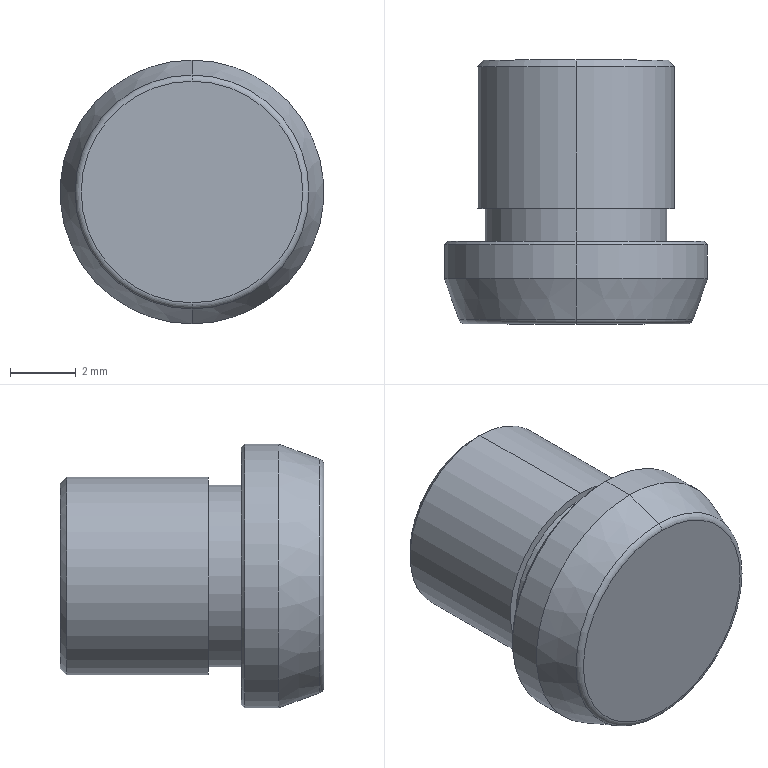Part | STEP file | BPSP-L-03 Fixture Locating Pin_Default | 1 solid | 18 faces | box 8 x 8 x 8 mm | volume 267.813 mm3 | cylinder 6 | cone 6 | plane 4 | torus 2 | commonest cylinder face diameters 5.5 x2 6 x2 8 x2
STEP:
#1=CARTESIAN_POINT('',(0.,0.,0.));
#2=DIRECTION('',(0.,0.,1.));
#3=DIRECTION('',(1.,0.,0.));
#4=AXIS2_PLACEMENT_3D('',#1,#2,#3);
#5=CARTESIAN_POINT('',(0.,7.8,-3.));
#6=VERTEX_POINT('',#5);
#7=CARTESIAN_POINT('',(0.,7.8,3.));
#8=VERTEX_POINT('',#7);
#9=CARTESIAN_POINT('',(0.,7.8,0.));
#10=DIRECTION('',(0.,-1.,0.));
#11=DIRECTION('',(0.,0.,1.));
#12=AXIS2_PLACEMENT_3D('',#9,#10,#11);
#13=CIRCLE('',#12,3.);
#14=CARTESIAN_POINT('',(0.,8.,0.));
#15=DIRECTION('',(0.,-1.,0.));
#16=DIRECTION('',(0.,0.,-1.));
#17=AXIS2_PLACEMENT_3D('',#14,#15,#16);
#18=CYLINDRICAL_SURFACE('',#17,3.);
#19=CARTESIAN_POINT('',(-3.142,0.2));
#20=DIRECTION('',(1.,0.));
#21=VECTOR('',#20,1.);
#22=LINE('',#19,#21);
#23=(GEOMETRIC_REPRESENTATION_CONTEXT(2)PARAMETRIC_REPRESENTATION_CONTEXT()REPRESENTATION_CONTEXT('',''));
#24=DEFINITIONAL_REPRESENTATION('',(#22),#23);
#25=PCURVE('',#18,#24);
#26=CARTESIAN_POINT('',(0.,8.,0.));
#27=DIRECTION('',(0.,-1.,0.));
#28=DIRECTION('',(0.,0.,-1.));
#29=AXIS2_PLACEMENT_3D('',#26,#27,#28);
#30=CONICAL_SURFACE('',#29,2.8,0.7854);
#31=CARTESIAN_POINT('',(-3.142,0.2));
#32=DIRECTION('',(1.,0.));
#33=VECTOR('',#32,1.);
#34=LINE('',#31,#33);
#35=(GEOMETRIC_REPRESENTATION_CONTEXT(2)PARAMETRIC_REPRESENTATION_CONTEXT()REPRESENTATION_CONTEXT('',''));
#36=DEFINITIONAL_REPRESENTATION('',(#34),#35);
#37=PCURVE('',#30,#36);
#38=SURFACE_CURVE('',#13,(#25,#37),.PCURVE_S1.);
#39=EDGE_CURVE('',#6,#8,#38,.T.);
#40=ORIENTED_EDGE('',*,*,#39,.T.);
#41=CARTESIAN_POINT('',(0.,3.5,3.));
#42=VERTEX_POINT('',#41);
#43=CARTESIAN_POINT('',(0.,8.,3.));
#44=DIRECTION('',(0.,-1.,0.));
#45=VECTOR('',#44,1.);
#46=LINE('',#43,#45);
#47=CARTESIAN_POINT('',(3.142,0.));
#48=DIRECTION('',(0.,1.));
#49=VECTOR('',#48,1.);
#50=LINE('',#47,#49);
#51=(GEOMETRIC_REPRESENTATION_CONTEXT(2)PARAMETRIC_REPRESENTATION_CONTEXT()REPRESENTATION_CONTEXT('',''));
#52=DEFINITIONAL_REPRESENTATION('',(#50),#51);
#53=PCURVE('',#18,#52);
#54=CARTESIAN_POINT('',(0.,8.,0.));
#55=DIRECTION('',(0.,-1.,0.));
#56=DIRECTION('',(0.,0.,-1.));
#57=AXIS2_PLACEMENT_3D('',#54,#55,#56);
#58=CYLINDRICAL_SURFACE('',#57,3.);
#59=CARTESIAN_POINT('',(3.142,0.));
#60=DIRECTION('',(0.,1.));
#61=VECTOR('',#60,1.);
#62=LINE('',#59,#61);
#63=(GEOMETRIC_REPRESENTATION_CONTEXT(2)PARAMETRIC_REPRESENTATION_CONTEXT()REPRESENTATION_CONTEXT('',''));
#64=DEFINITIONAL_REPRESENTATION('',(#62),#63);
#65=PCURVE('',#58,#64);
#66=SURFACE_CURVE('',#46,(#53,#65),.PCURVE_S1.);
#67=EDGE_CURVE('',#8,#42,#66,.T.);
#68=ORIENTED_EDGE('',*,*,#67,.T.);
#69=CARTESIAN_POINT('',(0.,3.5,-3.));
#70=VERTEX_POINT('',#69);
#71=CARTESIAN_POINT('',(0.,3.5,0.));
#72=DIRECTION('',(0.,1.,0.));
#73=DIRECTION('',(0.,0.,1.));
#74=AXIS2_PLACEMENT_3D('',#71,#72,#73);
#75=CIRCLE('',#74,3.);
#76=CARTESIAN_POINT('',(3.142,4.5));
#77=DIRECTION('',(-1.,0.));
#78=VECTOR('',#77,1.);
#79=LINE('',#76,#78);
#80=(GEOMETRIC_REPRESENTATION_CONTEXT(2)PARAMETRIC_REPRESENTATION_CONTEXT()REPRESENTATION_CONTEXT('',''));
#81=DEFINITIONAL_REPRESENTATION('',(#79),#80);
#82=PCURVE('',#18,#81);
#83=CARTESIAN_POINT('',(0.,3.5,0.));
#84=DIRECTION('',(0.,1.,0.));
#85=DIRECTION('',(0.,0.,1.));
#86=AXIS2_PLACEMENT_3D('',#83,#84,#85);
#87=PLANE('',#86);
#88=CARTESIAN_POINT('',(0.,0.));
#89=DIRECTION('',(1.,0.));
#90=AXIS2_PLACEMENT_2D('',#88,#89);
#91=CIRCLE('',#90,3.);
#92=(GEOMETRIC_REPRESENTATION_CONTEXT(2)PARAMETRIC_REPRESENTATION_CONTEXT()REPRESENTATION_CONTEXT('',''));
#93=DEFINITIONAL_REPRESENTATION('',(#91),#92);
#94=PCURVE('',#87,#93);
#95=SURFACE_CURVE('',#75,(#82,#94),.PCURVE_S1.);
#96=EDGE_CURVE('',#42,#70,#95,.T.);
#97=ORIENTED_EDGE('',*,*,#96,.T.);
#98=CARTESIAN_POINT('',(0.,8.,-3.));
#99=DIRECTION('',(0.,-1.,0.));
#100=VECTOR('',#99,1.);
#101=LINE('',#98,#100);
#102=CARTESIAN_POINT('',(0.,0.));
#103=DIRECTION('',(0.,1.));
#104=VECTOR('',#103,1.);
#105=LINE('',#102,#104);
#106=(GEOMETRIC_REPRESENTATION_CONTEXT(2)PARAMETRIC_REPRESENTATION_CONTEXT()REPRESENTATION_CONTEXT('',''));
#107=DEFINITIONAL_REPRESENTATION('',(#105),#106);
#108=PCURVE('',#18,#107);
#109=CARTESIAN_POINT('',(6.283,0.));
#110=DIRECTION('',(0.,1.));
#111=VECTOR('',#110,1.);
#112=LINE('',#109,#111);
#113=(GEOMETRIC_REPRESENTATION_CONTEXT(2)PARAMETRIC_REPRESENTATION_CONTEXT()REPRESENTATION_CONTEXT('',''));
#114=DEFINITIONAL_REPRESENTATION('',(#112),#113);
#115=PCURVE('',#58,#114);
#116=SURFACE_CURVE('',#101,(#108,#115),.PCURVE_S1.);
#117=EDGE_CURVE('',#6,#70,#116,.T.);
#118=ORIENTED_EDGE('',*,*,#117,.F.);
#119=EDGE_LOOP('',(#40,#68,#97,#118));
#120=FACE_BOUND('',#119,.T.);
#121=ADVANCED_FACE('',(#120),#18,.T.);
#122=CARTESIAN_POINT('',(0.,8.,2.8));
#123=VERTEX_POINT('',#122);
#124=CARTESIAN_POINT('',(0.,8.,-2.8));
#125=VERTEX_POINT('',#124);
#126=CARTESIAN_POINT('',(0.,8.,0.));
#127=DIRECTION('',(0.,1.,0.));
#128=DIRECTION('',(0.,0.,1.));
#129=AXIS2_PLACEMENT_3D('',#126,#127,#128);
#130=CIRCLE('',#129,2.8);
#131=CARTESIAN_POINT('',(3.142,0.));
#132=DIRECTION('',(-1.,0.));
#133=VECTOR('',#132,1.);
#134=LINE('',#131,#133);
#135=(GEOMETRIC_REPRESENTATION_CONTEXT(2)PARAMETRIC_REPRESENTATION_CONTEXT()REPRESENTATION_CONTEXT('',''));
#136=DEFINITIONAL_REPRESENTATION('',(#134),#135);
#137=PCURVE('',#30,#136);
#138=CARTESIAN_POINT('',(0.,8.,0.));
#139=DIRECTION('',(0.,1.,0.));
#140=DIRECTION('',(0.,0.,1.));
#141=AXIS2_PLACEMENT_3D('',#138,#139,#140);
#142=PLANE('',#141);
#143=CARTESIAN_POINT('',(0.,0.));
#144=DIRECTION('',(1.,0.));
#145=AXIS2_PLACEMENT_2D('',#143,#144);
#146=CIRCLE('',#145,2.8);
#147=(GEOMETRIC_REPRESENTATION_CONTEXT(2)PARAMETRIC_REPRESENTATION_CONTEXT()REPRESENTATION_CONTEXT('',''));
#148=DEFINITIONAL_REPRESENTATION('',(#146),#147);
#149=PCURVE('',#142,#148);
#150=SURFACE_CURVE('',#130,(#137,#149),.PCURVE_S1.);
#151=EDGE_CURVE('',#123,#125,#150,.T.);
#152=ORIENTED_EDGE('',*,*,#151,.F.);
#153=CARTESIAN_POINT('',(0.,8.,2.8));
#154=DIRECTION('',(0.,-0.7071,0.7071));
#155=VECTOR('',#154,1.);
#156=LINE('',#153,#155);
#157=CARTESIAN_POINT('',(3.142,0.));
#158=DIRECTION('',(0.,1.));
#159=VECTOR('',#158,1.);
#160=LINE('',#157,#159);
#161=(GEOMETRIC_REPRESENTATION_CONTEXT(2)PARAMETRIC_REPRESENTATION_CONTEXT()REPRESENTATION_CONTEXT('',''));
#162=DEFINITIONAL_REPRESENTATION('',(#160),#161);
#163=PCURVE('',#30,#162);
#164=CARTESIAN_POINT('',(0.,8.,0.));
#165=DIRECTION('',(0.,-1.,0.));
#166=DIRECTION('',(0.,0.,-1.));
#167=AXIS2_PLACEMENT_3D('',#164,#165,#166);
#168=CONICAL_SURFACE('',#167,2.8,0.7854);
#169=CARTESIAN_POINT('',(3.142,0.));
#170=DIRECTION('',(0.,1.));
#171=VECTOR('',#170,1.);
#172=LINE('',#169,#171);
#173=(GEOMETRIC_REPRESENTATION_CONTEXT(2)PARAMETRIC_REPRESENTATION_CONTEXT()REPRESENTATION_CONTEXT('',''));
#174=DEFINITIONAL_REPRESENTATION('',(#172),#173);
#175=PCURVE('',#168,#174);
#176=SURFACE_CURVE('',#156,(#163,#175),.PCURVE_S1.);
#177=EDGE_CURVE('',#123,#8,#176,.T.);
#178=ORIENTED_EDGE('',*,*,#177,.T.);
#179=ORIENTED_EDGE('',*,*,#39,.F.);
#180=CARTESIAN_POINT('',(0.,8.,-2.8));
#181=DIRECTION('',(0.,-0.7071,-0.7071));
#182=VECTOR('',#181,1.);
#183=LINE('',#180,#182);
#184=CARTESIAN_POINT('',(0.,0.));
#185=DIRECTION('',(0.,1.));
#186=VECTOR('',#185,1.);
#187=LINE('',#184,#186);
#188=(GEOMETRIC_REPRESENTATION_CONTEXT(2)PARAMETRIC_REPRESENTATION_CONTEXT()REPRESENTATION_CONTEXT('',''));
#189=DEFINITIONAL_REPRESENTATION('',(#187),#188);
#190=PCURVE('',#30,#189);
#191=CARTESIAN_POINT('',(6.283,0.));
#192=DIRECTION('',(0.,1.));
#193=VECTOR('',#192,1.);
#194=LINE('',#191,#193);
#195=(GEOMETRIC_REPRESENTATION_CONTEXT(2)PARAMETRIC_REPRESENTATION_CONTEXT()REPRESENTATION_CONTEXT('',''));
#196=DEFINITIONAL_REPRESENTATION('',(#194),#195);
#197=PCURVE('',#168,#196);
#198=SURFACE_CURVE('',#183,(#190,#197),.PCURVE_S1.);
#199=EDGE_CURVE('',#125,#6,#198,.T.);
#200=ORIENTED_EDGE('',*,*,#199,.F.);
#201=EDGE_LOOP('',(#152,#178,#179,#200));
#202=FACE_BOUND('',#201,.T.);
#203=ADVANCED_FACE('',(#202),#30,.T.);
#204=CARTESIAN_POINT('',(0.,3.5,2.75));
#205=VERTEX_POINT('',#204);
#206=CARTESIAN_POINT('',(0.,3.5,-2.75));
#207=VERTEX_POINT('',#206);
#208=CARTESIAN_POINT('',(0.,3.5,0.));
#209=DIRECTION('',(0.,1.,0.));
#210=DIRECTION('',(0.,0.,1.));
#211=AXIS2_PLACEMENT_3D('',#208,#209,#210);
#212=CIRCLE('',#211,2.75);
#213=CARTESIAN_POINT('',(0.,3.5,0.));
#214=DIRECTION('',(0.,-1.,0.));
#215=DIRECTION('',(0.,0.,-1.));
#216=AXIS2_PLACEMENT_3D('',#213,#214,#215);
#217=CYLINDRICAL_SURFACE('',#216,2.75);
#218=CARTESIAN_POINT('',(3.142,0.));
#219=DIRECTION('',(-1.,0.));
#220=VECTOR('',#219,1.);
#221=LINE('',#218,#220);
#222=(GEOMETRIC_REPRESENTATION_CONTEXT(2)PARAMETRIC_REPRESENTATION_CONTEXT()REPRESENTATION_CONTEXT('',''));
#223=DEFINITIONAL_REPRESENTATION('',(#221),#222);
#224=PCURVE('',#217,#223);
#225=CARTESIAN_POINT('',(0.,0.));
#226=DIRECTION('',(1.,0.));
#227=AXIS2_PLACEMENT_2D('',#225,#226);
#228=CIRCLE('',#227,2.75);
#229=(GEOMETRIC_REPRESENTATION_CONTEXT(2)PARAMETRIC_REPRESENTATION_CONTEXT()REPRESENTATION_CONTEXT('',''));
#230=DEFINITIONAL_REPRESENTATION('',(#228),#229);
#231=PCURVE('',#87,#230);
#232=SURFACE_CURVE('',#212,(#224,#231),.PCURVE_S1.);
#233=EDGE_CURVE('',#205,#207,#232,.T.);
#234=ORIENTED_EDGE('',*,*,#233,.F.);
#235=CARTESIAN_POINT('',(0.,2.5,2.75));
#236=VERTEX_POINT('',#235);
#237=CARTESIAN_POINT('',(0.,3.5,2.75));
#238=DIRECTION('',(0.,-1.,0.));
#239=VECTOR('',#238,1.);
#240=LINE('',#237,#239);
#241=CARTESIAN_POINT('',(3.142,0.));
#242=DIRECTION('',(0.,1.));
#243=VECTOR('',#242,1.);
#244=LINE('',#241,#243);
#245=(GEOMETRIC_REPRESENTATION_CONTEXT(2)PARAMETRIC_REPRESENTATION_CONTEXT()REPRESENTATION_CONTEXT('',''));
#246=DEFINITIONAL_REPRESENTATION('',(#244),#245);
#247=PCURVE('',#217,#246);
#248=CARTESIAN_POINT('',(0.,3.5,0.));
#249=DIRECTION('',(0.,-1.,0.));
#250=DIRECTION('',(0.,0.,-1.));
#251=AXIS2_PLACEMENT_3D('',#248,#249,#250);
#252=CYLINDRICAL_SURFACE('',#251,2.75);
#253=CARTESIAN_POINT('',(3.142,0.));
#254=DIRECTION('',(0.,1.));
#255=VECTOR('',#254,1.);
#256=LINE('',#253,#255);
#257=(GEOMETRIC_REPRESENTATION_CONTEXT(2)PARAMETRIC_REPRESENTATION_CONTEXT()REPRESENTATION_CONTEXT('',''));
#258=DEFINITIONAL_REPRESENTATION('',(#256),#257);
#259=PCURVE('',#252,#258);
#260=SURFACE_CURVE('',#240,(#247,#259),.PCURVE_S1.);
#261=EDGE_CURVE('',#205,#236,#260,.T.);
#262=ORIENTED_EDGE('',*,*,#261,.T.);
#263=CARTESIAN_POINT('',(0.,2.5,-2.75));
#264=VERTEX_POINT('',#263);
#265=CARTESIAN_POINT('',(0.,2.5,0.));
#266=DIRECTION('',(0.,1.,0.));
#267=DIRECTION('',(0.,0.,1.));
#268=AXIS2_PLACEMENT_3D('',#265,#266,#267);
#269=CIRCLE('',#268,2.75);
#270=CARTESIAN_POINT('',(3.142,1.));
#271=DIRECTION('',(-1.,0.));
#272=VECTOR('',#271,1.);
#273=LINE('',#270,#272);
#274=(GEOMETRIC_REPRESENTATION_CONTEXT(2)PARAMETRIC_REPRESENTATION_CONTEXT()REPRESENTATION_CONTEXT('',''));
#275=DEFINITIONAL_REPRESENTATION('',(#273),#274);
#276=PCURVE('',#217,#275);
#277=CARTESIAN_POINT('',(0.,2.5,0.));
#278=DIRECTION('',(0.,1.,0.));
#279=DIRECTION('',(0.,0.,1.));
#280=AXIS2_PLACEMENT_3D('',#277,#278,#279);
#281=PLANE('',#280);
#282=CARTESIAN_POINT('',(0.,0.));
#283=DIRECTION('',(1.,0.));
#284=AXIS2_PLACEMENT_2D('',#282,#283);
#285=CIRCLE('',#284,2.75);
#286=(GEOMETRIC_REPRESENTATION_CONTEXT(2)PARAMETRIC_REPRESENTATION_CONTEXT()REPRESENTATION_CONTEXT('',''));
#287=DEFINITIONAL_REPRESENTATION('',(#285),#286);
#288=PCURVE('',#281,#287);
#289=SURFACE_CURVE('',#269,(#276,#288),.PCURVE_S1.);
#290=EDGE_CURVE('',#236,#264,#289,.T.);
#291=ORIENTED_EDGE('',*,*,#290,.T.);
#292=CARTESIAN_POINT('',(0.,3.5,-2.75));
#293=DIRECTION('',(0.,-1.,0.));
#294=VECTOR('',#293,1.);
#295=LINE('',#292,#294);
#296=CARTESIAN_POINT('',(0.,0.));
#297=DIRECTION('',(0.,1.));
#298=VECTOR('',#297,1.);
#299=LINE('',#296,#298);
#300=(GEOMETRIC_REPRESENTATION_CONTEXT(2)PARAMETRIC_REPRESENTATION_CONTEXT()REPRESENTATION_CONTEXT('',''));
#301=DEFINITIONAL_REPRESENTATION('',(#299),#300);
#302=PCURVE('',#217,#301);
#303=CARTESIAN_POINT('',(6.283,0.));
#304=DIRECTION('',(0.,1.));
#305=VECTOR('',#304,1.);
#306=LINE('',#303,#305);
#307=(GEOMETRIC_REPRESENTATION_CONTEXT(2)PARAMETRIC_REPRESENTATION_CONTEXT()REPRESENTATION_CONTEXT('',''));
#308=DEFINITIONAL_REPRESENTATION('',(#306),#307);
#309=PCURVE('',#252,#308);
#310=SURFACE_CURVE('',#295,(#302,#309),.PCURVE_S1.);
#311=EDGE_CURVE('',#207,#264,#310,.T.);
#312=ORIENTED_EDGE('',*,*,#311,.F.);
#313=EDGE_LOOP('',(#234,#262,#291,#312));
#314=FACE_BOUND('',#313,.T.);
#315=ADVANCED_FACE('',(#314),#217,.T.);
#316=CARTESIAN_POINT('',(0.,0.,-3.36));
#317=VERTEX_POINT('',#316);
#318=CARTESIAN_POINT('',(0.,0.,3.36));
#319=VERTEX_POINT('',#318);
#320=CARTESIAN_POINT('',(0.,0.,0.));
#321=DIRECTION('',(0.,-1.,0.));
#322=DIRECTION('',(0.,0.,1.));
#323=AXIS2_PLACEMENT_3D('',#320,#321,#322);
#324=CIRCLE('',#323,3.36);
#325=CARTESIAN_POINT('',(0.,0.2,0.));
#326=DIRECTION('',(0.,1.,0.));
#327=DIRECTION('',(0.,0.,1.));
#328=AXIS2_PLACEMENT_3D('',#325,#326,#327);
#329=TOROIDAL_SURFACE('',#328,3.36,0.2);
#330=CARTESIAN_POINT('',(6.283,4.712));
#331=DIRECTION('',(-1.,0.));
#332=VECTOR('',#331,1.);
#333=LINE('',#330,#332);
#334=(GEOMETRIC_REPRESENTATION_CONTEXT(2)PARAMETRIC_REPRESENTATION_CONTEXT()REPRESENTATION_CONTEXT('',''));
#335=DEFINITIONAL_REPRESENTATION('',(#333),#334);
#336=PCURVE('',#329,#335);
#337=CARTESIAN_POINT('',(0.,0.,0.));
#338=DIRECTION('',(0.,1.,0.));
#339=DIRECTION('',(0.,0.,1.));
#340=AXIS2_PLACEMENT_3D('',#337,#338,#339);
#341=PLANE('',#340);
#342=CARTESIAN_POINT('',(3.36,0.));
#343=CARTESIAN_POINT('',(3.36,-5.82));
#344=CARTESIAN_POINT('',(-1.68,-2.91));
#345=CARTESIAN_POINT('',(-6.72,0.));
#346=CARTESIAN_POINT('',(-1.68,2.91));
#347=CARTESIAN_POINT('',(3.36,5.82));
#348=CARTESIAN_POINT('',(3.36,0.));
#349=(BOUNDED_CURVE()B_SPLINE_CURVE(2,(#342,#343,#344,#345,#346,#347,#348),.UNSPECIFIED.,.T.,.F.)B_SPLINE_CURVE_WITH_KNOTS((1,2,2,2,2,1),(-2.094,0.,2.094,4.189,6.283,8.378),.UNSPECIFIED.)CURVE()GEOMETRIC_REPRESENTATION_ITEM()RATIONAL_B_SPLINE_CURVE((1.,0.5,1.,0.5,1.,0.5,1.))REPRESENTATION_ITEM(''));
#350=(GEOMETRIC_REPRESENTATION_CONTEXT(2)PARAMETRIC_REPRESENTATION_CONTEXT()REPRESENTATION_CONTEXT('',''));
#351=DEFINITIONAL_REPRESENTATION('',(#349),#350);
#352=PCURVE('',#341,#351);
#353=SURFACE_CURVE('',#324,(#336,#352),.PCURVE_S1.);
#354=EDGE_CURVE('',#317,#319,#353,.T.);
#355=ORIENTED_EDGE('',*,*,#354,.F.);
#356=CARTESIAN_POINT('',(0.,0.1316,-3.548));
#357=VERTEX_POINT('',#356);
#358=CARTESIAN_POINT('',(0.,0.2,-3.36));
#359=DIRECTION('',(1.,0.,0.));
#360=DIRECTION('',(0.,0.,-1.));
#361=AXIS2_PLACEMENT_3D('',#358,#359,#360);
#362=CIRCLE('',#361,0.2);
#363=CARTESIAN_POINT('',(3.142,0.));
#364=DIRECTION('',(0.,1.));
#365=VECTOR('',#364,1.);
#366=LINE('',#363,#365);
#367=(GEOMETRIC_REPRESENTATION_CONTEXT(2)PARAMETRIC_REPRESENTATION_CONTEXT()REPRESENTATION_CONTEXT('',''));
#368=DEFINITIONAL_REPRESENTATION('',(#366),#367);
#369=PCURVE('',#329,#368);
#370=CARTESIAN_POINT('',(0.,0.2,0.));
#371=DIRECTION('',(0.,1.,0.));
#372=DIRECTION('',(0.,0.,1.));
#373=AXIS2_PLACEMENT_3D('',#370,#371,#372);
#374=TOROIDAL_SURFACE('',#373,3.36,0.2);
#375=CARTESIAN_POINT('',(3.142,0.));
#376=DIRECTION('',(0.,1.));
#377=VECTOR('',#376,1.);
#378=LINE('',#375,#377);
#379=(GEOMETRIC_REPRESENTATION_CONTEXT(2)PARAMETRIC_REPRESENTATION_CONTEXT()REPRESENTATION_CONTEXT('',''));
#380=DEFINITIONAL_REPRESENTATION('',(#378),#379);
#381=PCURVE('',#374,#380);
#382=SURFACE_CURVE('',#362,(#369,#381),.PCURVE_S1.);
#383=EDGE_CURVE('',#317,#357,#382,.T.);
#384=ORIENTED_EDGE('',*,*,#383,.T.);
#385=CARTESIAN_POINT('',(0.,0.1316,3.548));
#386=VERTEX_POINT('',#385);
#387=CARTESIAN_POINT('',(0.,0.1316,0.));
#388=DIRECTION('',(0.,1.,0.));
#389=DIRECTION('',(0.,0.,1.));
#390=AXIS2_PLACEMENT_3D('',#387,#388,#389);
#391=CIRCLE('',#390,3.548);
#392=CARTESIAN_POINT('',(0.,5.934));
#393=DIRECTION('',(1.,0.));
#394=VECTOR('',#393,1.);
#395=LINE('',#392,#394);
#396=(GEOMETRIC_REPRESENTATION_CONTEXT(2)PARAMETRIC_REPRESENTATION_CONTEXT()REPRESENTATION_CONTEXT('',''));
#397=DEFINITIONAL_REPRESENTATION('',(#395),#396);
#398=PCURVE('',#329,#397);
#399=CARTESIAN_POINT('',(0.,1.374,0.));
#400=DIRECTION('',(0.,1.,0.));
#401=DIRECTION('',(0.,0.,1.));
#402=AXIS2_PLACEMENT_3D('',#399,#400,#401);
#403=CONICAL_SURFACE('',#402,4.,0.3491);
#404=CARTESIAN_POINT('',(0.,-1.242));
#405=DIRECTION('',(1.,0.));
#406=VECTOR('',#405,1.);
#407=LINE('',#404,#406);
#408=(GEOMETRIC_REPRESENTATION_CONTEXT(2)PARAMETRIC_REPRESENTATION_CONTEXT()REPRESENTATION_CONTEXT('',''));
#409=DEFINITIONAL_REPRESENTATION('',(#407),#408);
#410=PCURVE('',#403,#409);
#411=SURFACE_CURVE('',#391,(#398,#410),.PCURVE_S1.);
#412=EDGE_CURVE('',#386,#357,#411,.T.);
#413=ORIENTED_EDGE('',*,*,#412,.F.);
#414=CARTESIAN_POINT('',(0.,0.2,3.36));
#415=DIRECTION('',(-1.,0.,0.));
#416=DIRECTION('',(0.,0.,1.));
#417=AXIS2_PLACEMENT_3D('',#414,#415,#416);
#418=CIRCLE('',#417,0.2);
#419=CARTESIAN_POINT('',(0.,0.));
#420=DIRECTION('',(0.,1.));
#421=VECTOR('',#420,1.);
#422=LINE('',#419,#421);
#423=(GEOMETRIC_REPRESENTATION_CONTEXT(2)PARAMETRIC_REPRESENTATION_CONTEXT()REPRESENTATION_CONTEXT('',''));
#424=DEFINITIONAL_REPRESENTATION('',(#422),#423);
#425=PCURVE('',#329,#424);
#426=CARTESIAN_POINT('',(6.283,0.));
#427=DIRECTION('',(0.,1.));
#428=VECTOR('',#427,1.);
#429=LINE('',#426,#428);
#430=(GEOMETRIC_REPRESENTATION_CONTEXT(2)PARAMETRIC_REPRESENTATION_CONTEXT()REPRESENTATION_CONTEXT('',''));
#431=DEFINITIONAL_REPRESENTATION('',(#429),#430);
#432=PCURVE('',#374,#431);
#433=SURFACE_CURVE('',#418,(#425,#432),.PCURVE_S1.);
#434=EDGE_CURVE('',#319,#386,#433,.T.);
#435=ORIENTED_EDGE('',*,*,#434,.F.);
#436=EDGE_LOOP('',(#355,#384,#413,#435));
#437=FACE_BOUND('',#436,.T.);
#438=ADVANCED_FACE('',(#437),#329,.T.);
#439=CARTESIAN_POINT('',(0.,2.5,3.9));
#440=VERTEX_POINT('',#439);
#441=CARTESIAN_POINT('',(0.,2.5,-3.9));
#442=VERTEX_POINT('',#441);
#443=CARTESIAN_POINT('',(0.,2.5,0.));
#444=DIRECTION('',(0.,1.,0.));
#445=DIRECTION('',(0.,0.,1.));
#446=AXIS2_PLACEMENT_3D('',#443,#444,#445);
#447=CIRCLE('',#446,3.9);
#448=CARTESIAN_POINT('',(0.,2.5,0.));
#449=DIRECTION('',(0.,-1.,0.));
#450=DIRECTION('',(0.,0.,-1.));
#451=AXIS2_PLACEMENT_3D('',#448,#449,#450);
#452=CONICAL_SURFACE('',#451,3.9,0.7854);
#453=CARTESIAN_POINT('',(3.142,0.));
#454=DIRECTION('',(-1.,0.));
#455=VECTOR('',#454,1.);
#456=LINE('',#453,#455);
#457=(GEOMETRIC_REPRESENTATION_CONTEXT(2)PARAMETRIC_REPRESENTATION_CONTEXT()REPRESENTATION_CONTEXT('',''));
#458=DEFINITIONAL_REPRESENTATION('',(#456),#457);
#459=PCURVE('',#452,#458);
#460=CARTESIAN_POINT('',(0.,0.));
#461=DIRECTION('',(1.,0.));
#462=AXIS2_PLACEMENT_2D('',#460,#461);
#463=CIRCLE('',#462,3.9);
#464=(GEOMETRIC_REPRESENTATION_CONTEXT(2)PARAMETRIC_REPRESENTATION_CONTEXT()REPRESENTATION_CONTEXT('',''));
#465=DEFINITIONAL_REPRESENTATION('',(#463),#464);
#466=PCURVE('',#281,#465);
#467=SURFACE_CURVE('',#447,(#459,#466),.PCURVE_S1.);
#468=EDGE_CURVE('',#440,#442,#467,.T.);
#469=ORIENTED_EDGE('',*,*,#468,.F.);
#470=CARTESIAN_POINT('',(0.,2.4,4.));
#471=VERTEX_POINT('',#470);
#472=CARTESIAN_POINT('',(0.,2.5,3.9));
#473=DIRECTION('',(0.,-0.7071,0.7071));
#474=VECTOR('',#473,1.);
#475=LINE('',#472,#474);
#476=CARTESIAN_POINT('',(3.142,0.));
#477=DIRECTION('',(0.,1.));
#478=VECTOR('',#477,1.);
#479=LINE('',#476,#478);
#480=(GEOMETRIC_REPRESENTATION_CONTEXT(2)PARAMETRIC_REPRESENTATION_CONTEXT()REPRESENTATION_CONTEXT('',''));
#481=DEFINITIONAL_REPRESENTATION('',(#479),#480);
#482=PCURVE('',#452,#481);
#483=CARTESIAN_POINT('',(0.,2.5,0.));
#484=DIRECTION('',(0.,-1.,0.));
#485=DIRECTION('',(0.,0.,-1.));
#486=AXIS2_PLACEMENT_3D('',#483,#484,#485);
#487=CONICAL_SURFACE('',#486,3.9,0.7854);
#488=CARTESIAN_POINT('',(3.142,0.));
#489=DIRECTION('',(0.,1.));
#490=VECTOR('',#489,1.);
#491=LINE('',#488,#490);
#492=(GEOMETRIC_REPRESENTATION_CONTEXT(2)PARAMETRIC_REPRESENTATION_CONTEXT()REPRESENTATION_CONTEXT('',''));
#493=DEFINITIONAL_REPRESENTATION('',(#491),#492);
#494=PCURVE('',#487,#493);
#495=SURFACE_CURVE('',#475,(#482,#494),.PCURVE_S1.);
#496=EDGE_CURVE('',#440,#471,#495,.T.);
#497=ORIENTED_EDGE('',*,*,#496,.T.);
#498=CARTESIAN_POINT('',(0.,2.4,-4.));
#499=VERTEX_POINT('',#498);
#500=CARTESIAN_POINT('',(0.,2.4,0.));
#501=DIRECTION('',(0.,-1.,0.));
#502=DIRECTION('',(0.,0.,1.));
#503=AXIS2_PLACEMENT_3D('',#500,#501,#502);
#504=CIRCLE('',#503,4.);
#505=CARTESIAN_POINT('',(-3.142,0.1));
#506=DIRECTION('',(1.,0.));
#507=VECTOR('',#506,1.);
#508=LINE('',#505,#507);
#509=(GEOMETRIC_REPRESENTATION_CONTEXT(2)PARAMETRIC_REPRESENTATION_CONTEXT()REPRESENTATION_CONTEXT('',''));
#510=DEFINITIONAL_REPRESENTATION('',(#508),#509);
#511=PCURVE('',#452,#510);
#512=CARTESIAN_POINT('',(0.,2.5,0.));
#513=DIRECTION('',(0.,-1.,0.));
#514=DIRECTION('',(0.,0.,-1.));
#515=AXIS2_PLACEMENT_3D('',#512,#513,#514);
#516=CYLINDRICAL_SURFACE('',#515,4.);
#517=CARTESIAN_POINT('',(-3.142,0.1));
#518=DIRECTION('',(1.,0.));
#519=VECTOR('',#518,1.);
#520=LINE('',#517,#519);
#521=(GEOMETRIC_REPRESENTATION_CONTEXT(2)PARAMETRIC_REPRESENTATION_CONTEXT()REPRESENTATION_CONTEXT('',''));
#522=DEFINITIONAL_REPRESENTATION('',(#520),#521);
#523=PCURVE('',#516,#522);
#524=SURFACE_CURVE('',#504,(#511,#523),.PCURVE_S1.);
#525=EDGE_CURVE('',#499,#471,#524,.T.);
#526=ORIENTED_EDGE('',*,*,#525,.F.);
#527=CARTESIAN_POINT('',(0.,2.5,-3.9));
#528=DIRECTION('',(0.,-0.7071,-0.7071));
#529=VECTOR('',#528,1.);
#530=LINE('',#527,#529);
#531=CARTESIAN_POINT('',(0.,0.));
#532=DIRECTION('',(0.,1.));
#533=VECTOR('',#532,1.);
#534=LINE('',#531,#533);
#535=(GEOMETRIC_REPRESENTATION_CONTEXT(2)PARAMETRIC_REPRESENTATION_CONTEXT()REPRESENTATION_CONTEXT('',''));
#536=DEFINITIONAL_REPRESENTATION('',(#534),#535);
#537=PCURVE('',#452,#536);
#538=CARTESIAN_POINT('',(6.283,0.));
#539=DIRECTION('',(0.,1.));
#540=VECTOR('',#539,1.);
#541=LINE('',#538,#540);
#542=(GEOMETRIC_REPRESENTATION_CONTEXT(2)PARAMETRIC_REPRESENTATION_CONTEXT()REPRESENTATION_CONTEXT('',''));
#543=DEFINITIONAL_REPRESENTATION('',(#541),#542);
#544=PCURVE('',#487,#543);
#545=SURFACE_CURVE('',#530,(#537,#544),.PCURVE_S1.);
#546=EDGE_CURVE('',#442,#499,#545,.T.);
#547=ORIENTED_EDGE('',*,*,#546,.F.);
#548=EDGE_LOOP('',(#469,#497,#526,#547));
#549=FACE_BOUND('',#548,.T.);
#550=ADVANCED_FACE('',(#549),#452,.T.);
#551=ORIENTED_EDGE('',*,*,#412,.T.);
#552=CARTESIAN_POINT('',(0.,1.374,-4.));
#553=VERTEX_POINT('',#552);
#554=CARTESIAN_POINT('',(0.,1.374,-4.));
#555=DIRECTION('',(0.,0.9397,-0.342));
#556=VECTOR('',#555,1.);
#557=LINE('',#554,#556);
#558=CARTESIAN_POINT('',(3.142,0.));
#559=DIRECTION('',(0.,1.));
#560=VECTOR('',#559,1.);
#561=LINE('',#558,#560);
#562=(GEOMETRIC_REPRESENTATION_CONTEXT(2)PARAMETRIC_REPRESENTATION_CONTEXT()REPRESENTATION_CONTEXT('',''));
#563=DEFINITIONAL_REPRESENTATION('',(#561),#562);
#564=PCURVE('',#403,#563);
#565=CARTESIAN_POINT('',(0.,1.374,0.));
#566=DIRECTION('',(0.,1.,0.));
#567=DIRECTION('',(0.,0.,1.));
#568=AXIS2_PLACEMENT_3D('',#565,#566,#567);
#569=CONICAL_SURFACE('',#568,4.,0.3491);
#570=CARTESIAN_POINT('',(3.142,0.));
#571=DIRECTION('',(0.,1.));
#572=VECTOR('',#571,1.);
#573=LINE('',#570,#572);
#574=(GEOMETRIC_REPRESENTATION_CONTEXT(2)PARAMETRIC_REPRESENTATION_CONTEXT()REPRESENTATION_CONTEXT('',''));
#575=DEFINITIONAL_REPRESENTATION('',(#573),#574);
#576=PCURVE('',#569,#575);
#577=SURFACE_CURVE('',#557,(#564,#576),.PCURVE_S1.);
#578=EDGE_CURVE('',#357,#553,#577,.T.);
#579=ORIENTED_EDGE('',*,*,#578,.T.);
#580=CARTESIAN_POINT('',(0.,1.374,4.));
#581=VERTEX_POINT('',#580);
#582=CARTESIAN_POINT('',(0.,1.374,0.));
#583=DIRECTION('',(0.,1.,0.));
#584=DIRECTION('',(0.,0.,1.));
#585=AXIS2_PLACEMENT_3D('',#582,#583,#584);
#586=CIRCLE('',#585,4.);
#587=CARTESIAN_POINT('',(0.,0.));
#588=DIRECTION('',(1.,0.));
#589=VECTOR('',#588,1.);
#590=LINE('',#587,#589);
#591=(GEOMETRIC_REPRESENTATION_CONTEXT(2)PARAMETRIC_REPRESENTATION_CONTEXT()REPRESENTATION_CONTEXT('',''));
#592=DEFINITIONAL_REPRESENTATION('',(#590),#591);
#593=PCURVE('',#403,#592);
#594=CARTESIAN_POINT('',(3.142,1.126));
#595=DIRECTION('',(-1.,0.));
#596=VECTOR('',#595,1.);
#597=LINE('',#594,#596);
#598=(GEOMETRIC_REPRESENTATION_CONTEXT(2)PARAMETRIC_REPRESENTATION_CONTEXT()REPRESENTATION_CONTEXT('',''));
#599=DEFINITIONAL_REPRESENTATION('',(#597),#598);
#600=PCURVE('',#516,#599);
#601=SURFACE_CURVE('',#586,(#593,#600),.PCURVE_S1.);
#602=EDGE_CURVE('',#581,#553,#601,.T.);
#603=ORIENTED_EDGE('',*,*,#602,.F.);
#604=CARTESIAN_POINT('',(0.,1.374,4.));
#605=DIRECTION('',(0.,0.9397,0.342));
#606=VECTOR('',#605,1.);
#607=LINE('',#604,#606);
#608=CARTESIAN_POINT('',(0.,0.));
#609=DIRECTION('',(0.,1.));
#610=VECTOR('',#609,1.);
#611=LINE('',#608,#610);
#612=(GEOMETRIC_REPRESENTATION_CONTEXT(2)PARAMETRIC_REPRESENTATION_CONTEXT()REPRESENTATION_CONTEXT('',''));
#613=DEFINITIONAL_REPRESENTATION('',(#611),#612);
#614=PCURVE('',#403,#613);
#615=CARTESIAN_POINT('',(6.283,0.));
#616=DIRECTION('',(0.,1.));
#617=VECTOR('',#616,1.);
#618=LINE('',#615,#617);
#619=(GEOMETRIC_REPRESENTATION_CONTEXT(2)PARAMETRIC_REPRESENTATION_CONTEXT()REPRESENTATION_CONTEXT('',''));
#620=DEFINITIONAL_REPRESENTATION('',(#618),#619);
#621=PCURVE('',#569,#620);
#622=SURFACE_CURVE('',#607,(#614,#621),.PCURVE_S1.);
#623=EDGE_CURVE('',#386,#581,#622,.T.);
#624=ORIENTED_EDGE('',*,*,#623,.F.);
#625=EDGE_LOOP('',(#551,#579,#603,#624));
#626=FACE_BOUND('',#625,.T.);
#627=ADVANCED_FACE('',(#626),#403,.T.);
#628=ORIENTED_EDGE('',*,*,#525,.T.);
#629=CARTESIAN_POINT('',(0.,2.5,4.));
#630=DIRECTION('',(0.,-1.,0.));
#631=VECTOR('',#630,1.);
#632=LINE('',#629,#631);
#633=CARTESIAN_POINT('',(3.142,0.));
#634=DIRECTION('',(0.,1.));
#635=VECTOR('',#634,1.);
#636=LINE('',#633,#635);
#637=(GEOMETRIC_REPRESENTATION_CONTEXT(2)PARAMETRIC_REPRESENTATION_CONTEXT()REPRESENTATION_CONTEXT('',''));
#638=DEFINITIONAL_REPRESENTATION('',(#636),#637);
#639=PCURVE('',#516,#638);
#640=CARTESIAN_POINT('',(0.,2.5,0.));
#641=DIRECTION('',(0.,-1.,0.));
#642=DIRECTION('',(0.,0.,-1.));
#643=AXIS2_PLACEMENT_3D('',#640,#641,#642);
#644=CYLINDRICAL_SURFACE('',#643,4.);
#645=CARTESIAN_POINT('',(3.142,0.));
#646=DIRECTION('',(0.,1.));
#647=VECTOR('',#646,1.);
#648=LINE('',#645,#647);
#649=(GEOMETRIC_REPRESENTATION_CONTEXT(2)PARAMETRIC_REPRESENTATION_CONTEXT()REPRESENTATION_CONTEXT('',''));
#650=DEFINITIONAL_REPRESENTATION('',(#648),#649);
#651=PCURVE('',#644,#650);
#652=SURFACE_CURVE('',#632,(#639,#651),.PCURVE_S1.);
#653=EDGE_CURVE('',#471,#581,#652,.T.);
#654=ORIENTED_EDGE('',*,*,#653,.T.);
#655=ORIENTED_EDGE('',*,*,#602,.T.);
#656=CARTESIAN_POINT('',(0.,2.5,-4.));
#657=DIRECTION('',(0.,-1.,0.));
#658=VECTOR('',#657,1.);
#659=LINE('',#656,#658);
#660=CARTESIAN_POINT('',(0.,0.));
#661=DIRECTION('',(0.,1.));
#662=VECTOR('',#661,1.);
#663=LINE('',#660,#662);
#664=(GEOMETRIC_REPRESENTATION_CONTEXT(2)PARAMETRIC_REPRESENTATION_CONTEXT()REPRESENTATION_CONTEXT('',''));
#665=DEFINITIONAL_REPRESENTATION('',(#663),#664);
#666=PCURVE('',#516,#665);
#667=CARTESIAN_POINT('',(6.283,0.));
#668=DIRECTION('',(0.,1.));
#669=VECTOR('',#668,1.);
#670=LINE('',#667,#669);
#671=(GEOMETRIC_REPRESENTATION_CONTEXT(2)PARAMETRIC_REPRESENTATION_CONTEXT()REPRESENTATION_CONTEXT('',''));
#672=DEFINITIONAL_REPRESENTATION('',(#670),#671);
#673=PCURVE('',#644,#672);
#674=SURFACE_CURVE('',#659,(#666,#673),.PCURVE_S1.);
#675=EDGE_CURVE('',#499,#553,#674,.T.);
#676=ORIENTED_EDGE('',*,*,#675,.F.);
#677=EDGE_LOOP('',(#628,#654,#655,#676));
#678=FACE_BOUND('',#677,.T.);
#679=ADVANCED_FACE('',(#678),#516,.T.);
#680=CARTESIAN_POINT('',(0.,2.5,0.));
#681=DIRECTION('',(0.,1.,0.));
#682=DIRECTION('',(0.,0.,1.));
#683=AXIS2_PLACEMENT_3D('',#680,#681,#682);
#684=CIRCLE('',#683,3.9);
#685=CARTESIAN_POINT('',(0.,0.));
#686=DIRECTION('',(1.,0.));
#687=AXIS2_PLACEMENT_2D('',#685,#686);
#688=CIRCLE('',#687,3.9);
#689=(GEOMETRIC_REPRESENTATION_CONTEXT(2)PARAMETRIC_REPRESENTATION_CONTEXT()REPRESENTATION_CONTEXT('',''));
#690=DEFINITIONAL_REPRESENTATION('',(#688),#689);
#691=PCURVE('',#281,#690);
#692=CARTESIAN_POINT('',(9.425,0.));
#693=DIRECTION('',(-1.,0.));
#694=VECTOR('',#693,1.);
#695=LINE('',#692,#694);
#696=(GEOMETRIC_REPRESENTATION_CONTEXT(2)PARAMETRIC_REPRESENTATION_CONTEXT()REPRESENTATION_CONTEXT('',''));
#697=DEFINITIONAL_REPRESENTATION('',(#695),#696);
#698=PCURVE('',#487,#697);
#699=SURFACE_CURVE('',#684,(#691,#698),.PCURVE_S1.);
#700=EDGE_CURVE('',#442,#440,#699,.T.);
#701=ORIENTED_EDGE('',*,*,#700,.T.);
#702=ORIENTED_EDGE('',*,*,#468,.T.);
#703=EDGE_LOOP('',(#701,#702));
#704=FACE_BOUND('',#703,.T.);
#705=CARTESIAN_POINT('',(0.,2.5,0.));
#706=DIRECTION('',(0.,1.,0.));
#707=DIRECTION('',(0.,0.,1.));
#708=AXIS2_PLACEMENT_3D('',#705,#706,#707);
#709=CIRCLE('',#708,2.75);
#710=CARTESIAN_POINT('',(0.,0.));
#711=DIRECTION('',(1.,0.));
#712=AXIS2_PLACEMENT_2D('',#710,#711);
#713=CIRCLE('',#712,2.75);
#714=(GEOMETRIC_REPRESENTATION_CONTEXT(2)PARAMETRIC_REPRESENTATION_CONTEXT()REPRESENTATION_CONTEXT('',''));
#715=DEFINITIONAL_REPRESENTATION('',(#713),#714);
#716=PCURVE('',#281,#715);
#717=CARTESIAN_POINT('',(9.425,1.));
#718=DIRECTION('',(-1.,0.));
#719=VECTOR('',#718,1.);
#720=LINE('',#717,#719);
#721=(GEOMETRIC_REPRESENTATION_CONTEXT(2)PARAMETRIC_REPRESENTATION_CONTEXT()REPRESENTATION_CONTEXT('',''));
#722=DEFINITIONAL_REPRESENTATION('',(#720),#721);
#723=PCURVE('',#252,#722);
#724=SURFACE_CURVE('',#709,(#716,#723),.PCURVE_S1.);
#725=EDGE_CURVE('',#264,#236,#724,.T.);
#726=ORIENTED_EDGE('',*,*,#725,.F.);
#727=ORIENTED_EDGE('',*,*,#290,.F.);
#728=EDGE_LOOP('',(#726,#727));
#729=FACE_BOUND('',#728,.T.);
#730=ADVANCED_FACE('',(#704,#729),#281,.T.);
#731=ORIENTED_EDGE('',*,*,#653,.F.);
#732=CARTESIAN_POINT('',(0.,2.4,0.));
#733=DIRECTION('',(0.,-1.,0.));
#734=DIRECTION('',(0.,0.,1.));
#735=AXIS2_PLACEMENT_3D('',#732,#733,#734);
#736=CIRCLE('',#735,4.);
#737=CARTESIAN_POINT('',(3.142,0.1));
#738=DIRECTION('',(1.,0.));
#739=VECTOR('',#738,1.);
#740=LINE('',#737,#739);
#741=(GEOMETRIC_REPRESENTATION_CONTEXT(2)PARAMETRIC_REPRESENTATION_CONTEXT()REPRESENTATION_CONTEXT('',''));
#742=DEFINITIONAL_REPRESENTATION('',(#740),#741);
#743=PCURVE('',#644,#742);
#744=CARTESIAN_POINT('',(3.142,0.1));
#745=DIRECTION('',(1.,0.));
#746=VECTOR('',#745,1.);
#747=LINE('',#744,#746);
#748=(GEOMETRIC_REPRESENTATION_CONTEXT(2)PARAMETRIC_REPRESENTATION_CONTEXT()REPRESENTATION_CONTEXT('',''));
#749=DEFINITIONAL_REPRESENTATION('',(#747),#748);
#750=PCURVE('',#487,#749);
#751=SURFACE_CURVE('',#736,(#743,#750),.PCURVE_S1.);
#752=EDGE_CURVE('',#471,#499,#751,.T.);
#753=ORIENTED_EDGE('',*,*,#752,.T.);
#754=ORIENTED_EDGE('',*,*,#675,.T.);
#755=CARTESIAN_POINT('',(0.,1.374,0.));
#756=DIRECTION('',(0.,1.,0.));
#757=DIRECTION('',(0.,0.,1.));
#758=AXIS2_PLACEMENT_3D('',#755,#756,#757);
#759=CIRCLE('',#758,4.);
#760=CARTESIAN_POINT('',(9.425,1.126));
#761=DIRECTION('',(-1.,0.));
#762=VECTOR('',#761,1.);
#763=LINE('',#760,#762);
#764=(GEOMETRIC_REPRESENTATION_CONTEXT(2)PARAMETRIC_REPRESENTATION_CONTEXT()REPRESENTATION_CONTEXT('',''));
#765=DEFINITIONAL_REPRESENTATION('',(#763),#764);
#766=PCURVE('',#644,#765);
#767=CARTESIAN_POINT('',(0.,0.));
#768=DIRECTION('',(1.,0.));
#769=VECTOR('',#768,1.);
#770=LINE('',#767,#769);
#771=(GEOMETRIC_REPRESENTATION_CONTEXT(2)PARAMETRIC_REPRESENTATION_CONTEXT()REPRESENTATION_CONTEXT('',''));
#772=DEFINITIONAL_REPRESENTATION('',(#770),#771);
#773=PCURVE('',#569,#772);
#774=SURFACE_CURVE('',#759,(#766,#773),.PCURVE_S1.);
#775=EDGE_CURVE('',#553,#581,#774,.T.);
#776=ORIENTED_EDGE('',*,*,#775,.T.);
#777=EDGE_LOOP('',(#731,#753,#754,#776));
#778=FACE_BOUND('',#777,.T.);
#779=ADVANCED_FACE('',(#778),#644,.T.);
#780=CARTESIAN_POINT('',(0.,0.,0.));
#781=DIRECTION('',(0.,-1.,0.));
#782=DIRECTION('',(0.,0.,1.));
#783=AXIS2_PLACEMENT_3D('',#780,#781,#782);
#784=CIRCLE('',#783,3.36);
#785=CARTESIAN_POINT('',(3.36,0.));
#786=CARTESIAN_POINT('',(3.36,-5.82));
#787=CARTESIAN_POINT('',(-1.68,-2.91));
#788=CARTESIAN_POINT('',(-6.72,0.));
#789=CARTESIAN_POINT('',(-1.68,2.91));
#790=CARTESIAN_POINT('',(3.36,5.82));
#791=CARTESIAN_POINT('',(3.36,0.));
#792=(BOUNDED_CURVE()B_SPLINE_CURVE(2,(#785,#786,#787,#788,#789,#790,#791),.UNSPECIFIED.,.T.,.F.)B_SPLINE_CURVE_WITH_KNOTS((1,2,2,2,2,1),(-2.094,0.,2.094,4.189,6.283,8.378),.UNSPECIFIED.)CURVE()GEOMETRIC_REPRESENTATION_ITEM()RATIONAL_B_SPLINE_CURVE((1.,0.5,1.,0.5,1.,0.5,1.))REPRESENTATION_ITEM(''));
#793=(GEOMETRIC_REPRESENTATION_CONTEXT(2)PARAMETRIC_REPRESENTATION_CONTEXT()REPRESENTATION_CONTEXT('',''));
#794=DEFINITIONAL_REPRESENTATION('',(#792),#793);
#795=PCURVE('',#341,#794);
#796=CARTESIAN_POINT('',(6.283,4.712));
#797=DIRECTION('',(-1.,0.));
#798=VECTOR('',#797,1.);
#799=LINE('',#796,#798);
#800=(GEOMETRIC_REPRESENTATION_CONTEXT(2)PARAMETRIC_REPRESENTATION_CONTEXT()REPRESENTATION_CONTEXT('',''));
#801=DEFINITIONAL_REPRESENTATION('',(#799),#800);
#802=PCURVE('',#374,#801);
#803=SURFACE_CURVE('',#784,(#795,#802),.PCURVE_S1.);
#804=EDGE_CURVE('',#319,#317,#803,.T.);
#805=ORIENTED_EDGE('',*,*,#804,.T.);
#806=ORIENTED_EDGE('',*,*,#354,.T.);
#807=EDGE_LOOP('',(#805,#806));
#808=FACE_BOUND('',#807,.T.);
#809=ADVANCED_FACE('',(#808),#341,.F.);
#810=ORIENTED_EDGE('',*,*,#578,.F.);
#811=CARTESIAN_POINT('',(0.,0.1316,0.));
#812=DIRECTION('',(0.,1.,0.));
#813=DIRECTION('',(0.,0.,1.));
#814=AXIS2_PLACEMENT_3D('',#811,#812,#813);
#815=CIRCLE('',#814,3.548);
#816=CARTESIAN_POINT('',(0.,-1.242));
#817=DIRECTION('',(1.,0.));
#818=VECTOR('',#817,1.);
#819=LINE('',#816,#818);
#820=(GEOMETRIC_REPRESENTATION_CONTEXT(2)PARAMETRIC_REPRESENTATION_CONTEXT()REPRESENTATION_CONTEXT('',''));
#821=DEFINITIONAL_REPRESENTATION('',(#819),#820);
#822=PCURVE('',#569,#821);
#823=CARTESIAN_POINT('',(0.,5.934));
#824=DIRECTION('',(1.,0.));
#825=VECTOR('',#824,1.);
#826=LINE('',#823,#825);
#827=(GEOMETRIC_REPRESENTATION_CONTEXT(2)PARAMETRIC_REPRESENTATION_CONTEXT()REPRESENTATION_CONTEXT('',''));
#828=DEFINITIONAL_REPRESENTATION('',(#826),#827);
#829=PCURVE('',#374,#828);
#830=SURFACE_CURVE('',#815,(#822,#829),.PCURVE_S1.);
#831=EDGE_CURVE('',#357,#386,#830,.T.);
#832=ORIENTED_EDGE('',*,*,#831,.T.);
#833=ORIENTED_EDGE('',*,*,#623,.T.);
#834=ORIENTED_EDGE('',*,*,#775,.F.);
#835=EDGE_LOOP('',(#810,#832,#833,#834));
#836=FACE_BOUND('',#835,.T.);
#837=ADVANCED_FACE('',(#836),#569,.T.);
#838=ORIENTED_EDGE('',*,*,#496,.F.);
#839=ORIENTED_EDGE('',*,*,#700,.F.);
#840=ORIENTED_EDGE('',*,*,#546,.T.);
#841=ORIENTED_EDGE('',*,*,#752,.F.);
#842=EDGE_LOOP('',(#838,#839,#840,#841));
#843=FACE_BOUND('',#842,.T.);
#844=ADVANCED_FACE('',(#843),#487,.T.);
#845=ORIENTED_EDGE('',*,*,#383,.F.);
#846=ORIENTED_EDGE('',*,*,#804,.F.);
#847=ORIENTED_EDGE('',*,*,#434,.T.);
#848=ORIENTED_EDGE('',*,*,#831,.F.);
#849=EDGE_LOOP('',(#845,#846,#847,#848));
#850=FACE_BOUND('',#849,.T.);
#851=ADVANCED_FACE('',(#850),#374,.T.);
#852=CARTESIAN_POINT('',(0.,3.5,0.));
#853=DIRECTION('',(0.,1.,0.));
#854=DIRECTION('',(0.,0.,1.));
#855=AXIS2_PLACEMENT_3D('',#852,#853,#854);
#856=CIRCLE('',#855,2.75);
#857=CARTESIAN_POINT('',(0.,0.));
#858=DIRECTION('',(1.,0.));
#859=AXIS2_PLACEMENT_2D('',#857,#858);
#860=CIRCLE('',#859,2.75);
#861=(GEOMETRIC_REPRESENTATION_CONTEXT(2)PARAMETRIC_REPRESENTATION_CONTEXT()REPRESENTATION_CONTEXT('',''));
#862=DEFINITIONAL_REPRESENTATION('',(#860),#861);
#863=PCURVE('',#87,#862);
#864=CARTESIAN_POINT('',(9.425,0.));
#865=DIRECTION('',(-1.,0.));
#866=VECTOR('',#865,1.);
#867=LINE('',#864,#866);
#868=(GEOMETRIC_REPRESENTATION_CONTEXT(2)PARAMETRIC_REPRESENTATION_CONTEXT()REPRESENTATION_CONTEXT('',''));
#869=DEFINITIONAL_REPRESENTATION('',(#867),#868);
#870=PCURVE('',#252,#869);
#871=SURFACE_CURVE('',#856,(#863,#870),.PCURVE_S1.);
#872=EDGE_CURVE('',#207,#205,#871,.T.);
#873=ORIENTED_EDGE('',*,*,#872,.T.);
#874=ORIENTED_EDGE('',*,*,#233,.T.);
#875=EDGE_LOOP('',(#873,#874));
#876=FACE_BOUND('',#875,.T.);
#877=CARTESIAN_POINT('',(0.,3.5,0.));
#878=DIRECTION('',(0.,1.,0.));
#879=DIRECTION('',(0.,0.,1.));
#880=AXIS2_PLACEMENT_3D('',#877,#878,#879);
#881=CIRCLE('',#880,3.);
#882=CARTESIAN_POINT('',(0.,0.));
#883=DIRECTION('',(1.,0.));
#884=AXIS2_PLACEMENT_2D('',#882,#883);
#885=CIRCLE('',#884,3.);
#886=(GEOMETRIC_REPRESENTATION_CONTEXT(2)PARAMETRIC_REPRESENTATION_CONTEXT()REPRESENTATION_CONTEXT('',''));
#887=DEFINITIONAL_REPRESENTATION('',(#885),#886);
#888=PCURVE('',#87,#887);
#889=CARTESIAN_POINT('',(9.425,4.5));
#890=DIRECTION('',(-1.,0.));
#891=VECTOR('',#890,1.);
#892=LINE('',#889,#891);
#893=(GEOMETRIC_REPRESENTATION_CONTEXT(2)PARAMETRIC_REPRESENTATION_CONTEXT()REPRESENTATION_CONTEXT('',''));
#894=DEFINITIONAL_REPRESENTATION('',(#892),#893);
#895=PCURVE('',#58,#894);
#896=SURFACE_CURVE('',#881,(#888,#895),.PCURVE_S1.);
#897=EDGE_CURVE('',#70,#42,#896,.T.);
#898=ORIENTED_EDGE('',*,*,#897,.F.);
#899=ORIENTED_EDGE('',*,*,#96,.F.);
#900=EDGE_LOOP('',(#898,#899));
#901=FACE_BOUND('',#900,.T.);
#902=ADVANCED_FACE('',(#876,#901),#87,.F.);
#903=ORIENTED_EDGE('',*,*,#261,.F.);
#904=ORIENTED_EDGE('',*,*,#872,.F.);
#905=ORIENTED_EDGE('',*,*,#311,.T.);
#906=ORIENTED_EDGE('',*,*,#725,.T.);
#907=EDGE_LOOP('',(#903,#904,#905,#906));
#908=FACE_BOUND('',#907,.T.);
#909=ADVANCED_FACE('',(#908),#252,.T.);
#910=CARTESIAN_POINT('',(0.,8.,0.));
#911=DIRECTION('',(0.,1.,0.));
#912=DIRECTION('',(0.,0.,1.));
#913=AXIS2_PLACEMENT_3D('',#910,#911,#912);
#914=CIRCLE('',#913,2.8);
#915=CARTESIAN_POINT('',(0.,0.));
#916=DIRECTION('',(1.,0.));
#917=AXIS2_PLACEMENT_2D('',#915,#916);
#918=CIRCLE('',#917,2.8);
#919=(GEOMETRIC_REPRESENTATION_CONTEXT(2)PARAMETRIC_REPRESENTATION_CONTEXT()REPRESENTATION_CONTEXT('',''));
#920=DEFINITIONAL_REPRESENTATION('',(#918),#919);
#921=PCURVE('',#142,#920);
#922=CARTESIAN_POINT('',(9.425,0.));
#923=DIRECTION('',(-1.,0.));
#924=VECTOR('',#923,1.);
#925=LINE('',#922,#924);
#926=(GEOMETRIC_REPRESENTATION_CONTEXT(2)PARAMETRIC_REPRESENTATION_CONTEXT()REPRESENTATION_CONTEXT('',''));
#927=DEFINITIONAL_REPRESENTATION('',(#925),#926);
#928=PCURVE('',#168,#927);
#929=SURFACE_CURVE('',#914,(#921,#928),.PCURVE_S1.);
#930=EDGE_CURVE('',#125,#123,#929,.T.);
#931=ORIENTED_EDGE('',*,*,#930,.T.);
#932=ORIENTED_EDGE('',*,*,#151,.T.);
#933=EDGE_LOOP('',(#931,#932));
#934=FACE_BOUND('',#933,.T.);
#935=ADVANCED_FACE('',(#934),#142,.T.);
#936=ORIENTED_EDGE('',*,*,#177,.F.);
#937=ORIENTED_EDGE('',*,*,#930,.F.);
#938=ORIENTED_EDGE('',*,*,#199,.T.);
#939=CARTESIAN_POINT('',(0.,7.8,0.));
#940=DIRECTION('',(0.,-1.,0.));
#941=DIRECTION('',(0.,0.,1.));
#942=AXIS2_PLACEMENT_3D('',#939,#940,#941);
#943=CIRCLE('',#942,3.);
#944=CARTESIAN_POINT('',(3.142,0.2));
#945=DIRECTION('',(1.,0.));
#946=VECTOR('',#945,1.);
#947=LINE('',#944,#946);
#948=(GEOMETRIC_REPRESENTATION_CONTEXT(2)PARAMETRIC_REPRESENTATION_CONTEXT()REPRESENTATION_CONTEXT('',''));
#949=DEFINITIONAL_REPRESENTATION('',(#947),#948);
#950=PCURVE('',#168,#949);
#951=CARTESIAN_POINT('',(3.142,0.2));
#952=DIRECTION('',(1.,0.));
#953=VECTOR('',#952,1.);
#954=LINE('',#951,#953);
#955=(GEOMETRIC_REPRESENTATION_CONTEXT(2)PARAMETRIC_REPRESENTATION_CONTEXT()REPRESENTATION_CONTEXT('',''));
#956=DEFINITIONAL_REPRESENTATION('',(#954),#955);
#957=PCURVE('',#58,#956);
#958=SURFACE_CURVE('',#943,(#950,#957),.PCURVE_S1.);
#959=EDGE_CURVE('',#8,#6,#958,.T.);
#960=ORIENTED_EDGE('',*,*,#959,.F.);
#961=EDGE_LOOP('',(#936,#937,#938,#960));
#962=FACE_BOUND('',#961,.T.);
#963=ADVANCED_FACE('',(#962),#168,.T.);
#964=ORIENTED_EDGE('',*,*,#67,.F.);
#965=ORIENTED_EDGE('',*,*,#959,.T.);
#966=ORIENTED_EDGE('',*,*,#117,.T.);
#967=ORIENTED_EDGE('',*,*,#897,.T.);
#968=EDGE_LOOP('',(#964,#965,#966,#967));
#969=FACE_BOUND('',#968,.T.);
#970=ADVANCED_FACE('',(#969),#58,.T.);
#971=CLOSED_SHELL('',(#121,#203,#315,#438,#550,#627,#679,#730,#779,#809,#837,#844,#851,#902,#909,#935,#963,#970));
#972=MANIFOLD_SOLID_BREP('',#971);
#973=(LENGTH_UNIT()NAMED_UNIT(*)SI_UNIT(.MILLI.,.METRE.));
#974=UNCERTAINTY_MEASURE_WITH_UNIT(LENGTH_MEASURE(0.0000001),#973,'','');
#975=(NAMED_UNIT(*)PLANE_ANGLE_UNIT()SI_UNIT($,.RADIAN.));
#976=(NAMED_UNIT(*)SI_UNIT($,.STERADIAN.)SOLID_ANGLE_UNIT());
#977=(GEOMETRIC_REPRESENTATION_CONTEXT(3)GLOBAL_UNCERTAINTY_ASSIGNED_CONTEXT((#974))GLOBAL_UNIT_ASSIGNED_CONTEXT((#973,#975,#976))REPRESENTATION_CONTEXT('',''));
#978=ADVANCED_BREP_SHAPE_REPRESENTATION('',(#4,#972),#977);